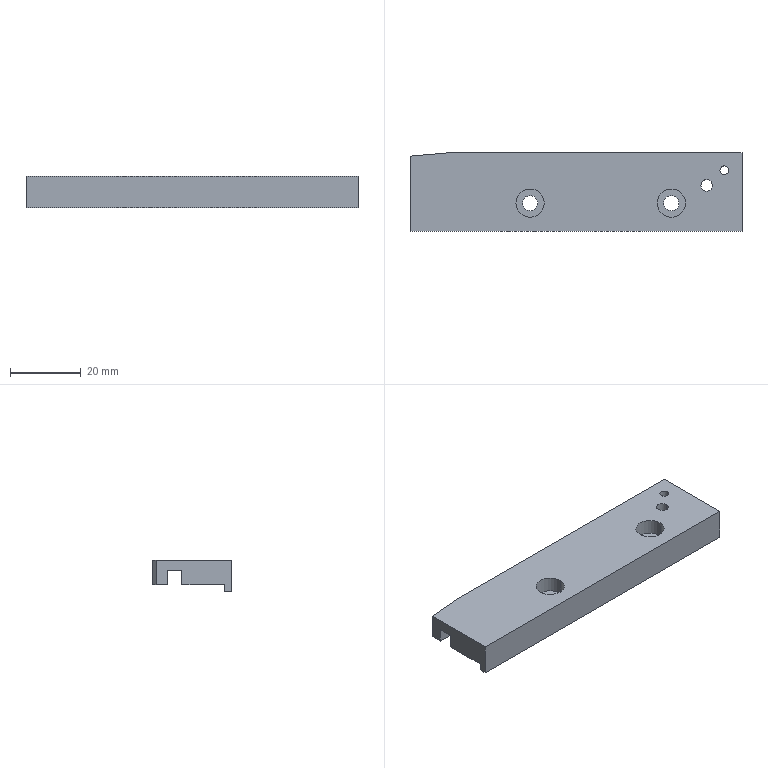Part | NX | features BREP 1 | 1 solid | 29 faces | box 94 x 22.3 x 9 mm | volume 12915 mm3 | plane 17 | cylinder 12 | commonest cylinder face diameters 4.3 x4 8 x4 2.5 x2 3.3 x2
STEP:
#1=CARTESIAN_POINT('',(33.75,6.15,4.));
#2=VERTEX_POINT('',#1);
#3=CARTESIAN_POINT('',(36.25,6.15,4.));
#4=VERTEX_POINT('',#3);
#5=CARTESIAN_POINT('',(35.,6.15,4.));
#6=DIRECTION('',(0.,0.,1.));
#7=DIRECTION('',(1.,0.,0.));
#8=AXIS2_PLACEMENT_3D('',#5,#6,#7);
#9=CIRCLE('',#8,1.25);
#10=EDGE_CURVE('',#2,#4,#9,.T.);
#11=ORIENTED_EDGE('',*,*,#10,.F.);
#12=CARTESIAN_POINT('',(33.75,6.15,7.));
#13=VERTEX_POINT('',#12);
#14=CARTESIAN_POINT('',(33.75,6.15,7.));
#15=DIRECTION('',(0.,0.,1.));
#16=VECTOR('',#15,1000.);
#17=LINE('',#14,#16);
#18=EDGE_CURVE('',#13,#2,#17,.F.);
#19=ORIENTED_EDGE('',*,*,#18,.F.);
#20=CARTESIAN_POINT('',(36.25,6.15,7.));
#21=VERTEX_POINT('',#20);
#22=CARTESIAN_POINT('',(35.,6.15,7.));
#23=DIRECTION('',(0.,0.,1.));
#24=DIRECTION('',(1.,0.,0.));
#25=AXIS2_PLACEMENT_3D('',#22,#23,#24);
#26=CIRCLE('',#25,1.25);
#27=EDGE_CURVE('',#13,#21,#26,.T.);
#28=ORIENTED_EDGE('',*,*,#27,.T.);
#29=CARTESIAN_POINT('',(36.25,6.15,7.));
#30=DIRECTION('',(0.,0.,1.));
#31=VECTOR('',#30,1000.);
#32=LINE('',#29,#31);
#33=EDGE_CURVE('',#21,#4,#32,.F.);
#34=ORIENTED_EDGE('',*,*,#33,.T.);
#35=EDGE_LOOP('',(#11,#19,#28,#34));
#36=FACE_BOUND('',#35,.T.);
#37=CARTESIAN_POINT('',(35.,6.15,7.));
#38=DIRECTION('',(0.,0.,1.));
#39=DIRECTION('',(1.,0.,0.));
#40=AXIS2_PLACEMENT_3D('',#37,#38,#39);
#41=CYLINDRICAL_SURFACE('',#40,1.25);
#42=ADVANCED_FACE('',(#36),#41,.F.);
#43=CARTESIAN_POINT('',(31.65,1.85,0.));
#44=VERTEX_POINT('',#43);
#45=CARTESIAN_POINT('',(28.35,1.85,0.));
#46=VERTEX_POINT('',#45);
#47=CARTESIAN_POINT('',(30.,1.85,0.));
#48=DIRECTION('',(0.,0.,-1.));
#49=DIRECTION('',(-1.,0.,0.));
#50=AXIS2_PLACEMENT_3D('',#47,#48,#49);
#51=CIRCLE('',#50,1.65);
#52=EDGE_CURVE('',#44,#46,#51,.T.);
#53=ORIENTED_EDGE('',*,*,#52,.T.);
#54=CARTESIAN_POINT('',(28.35,1.85,7.));
#55=VERTEX_POINT('',#54);
#56=CARTESIAN_POINT('',(28.35,1.85,7.));
#57=DIRECTION('',(0.,0.,1.));
#58=VECTOR('',#57,1000.);
#59=LINE('',#56,#58);
#60=EDGE_CURVE('',#55,#46,#59,.F.);
#61=ORIENTED_EDGE('',*,*,#60,.F.);
#62=CARTESIAN_POINT('',(31.65,1.85,7.));
#63=VERTEX_POINT('',#62);
#64=CARTESIAN_POINT('',(30.,1.85,7.));
#65=DIRECTION('',(0.,0.,1.));
#66=DIRECTION('',(1.,0.,0.));
#67=AXIS2_PLACEMENT_3D('',#64,#65,#66);
#68=CIRCLE('',#67,1.65);
#69=EDGE_CURVE('',#55,#63,#68,.T.);
#70=ORIENTED_EDGE('',*,*,#69,.T.);
#71=CARTESIAN_POINT('',(31.65,1.85,7.));
#72=DIRECTION('',(0.,0.,1.));
#73=VECTOR('',#72,1000.);
#74=LINE('',#71,#73);
#75=EDGE_CURVE('',#63,#44,#74,.F.);
#76=ORIENTED_EDGE('',*,*,#75,.T.);
#77=EDGE_LOOP('',(#53,#61,#70,#76));
#78=FACE_BOUND('',#77,.T.);
#79=CARTESIAN_POINT('',(30.,1.85,7.));
#80=DIRECTION('',(0.,0.,1.));
#81=DIRECTION('',(1.,0.,0.));
#82=AXIS2_PLACEMENT_3D('',#79,#80,#81);
#83=CYLINDRICAL_SURFACE('',#82,1.65);
#84=ADVANCED_FACE('',(#78),#83,.F.);
#85=CARTESIAN_POINT('',(16.,-3.15,2.6));
#86=VERTEX_POINT('',#85);
#87=CARTESIAN_POINT('',(24.,-3.15,2.6));
#88=VERTEX_POINT('',#87);
#89=CARTESIAN_POINT('',(20.,-3.15,2.6));
#90=DIRECTION('',(0.,0.,1.));
#91=DIRECTION('',(1.,0.,0.));
#92=AXIS2_PLACEMENT_3D('',#89,#90,#91);
#93=CIRCLE('',#92,4.);
#94=EDGE_CURVE('',#86,#88,#93,.T.);
#95=ORIENTED_EDGE('',*,*,#94,.F.);
#96=CARTESIAN_POINT('',(16.,-3.15,7.));
#97=VERTEX_POINT('',#96);
#98=CARTESIAN_POINT('',(16.,-3.15,7.));
#99=DIRECTION('',(0.,0.,1.));
#100=VECTOR('',#99,1000.);
#101=LINE('',#98,#100);
#102=EDGE_CURVE('',#97,#86,#101,.F.);
#103=ORIENTED_EDGE('',*,*,#102,.F.);
#104=CARTESIAN_POINT('',(24.,-3.15,7.));
#105=VERTEX_POINT('',#104);
#106=CARTESIAN_POINT('',(20.,-3.15,7.));
#107=DIRECTION('',(0.,0.,1.));
#108=DIRECTION('',(1.,0.,0.));
#109=AXIS2_PLACEMENT_3D('',#106,#107,#108);
#110=CIRCLE('',#109,4.);
#111=EDGE_CURVE('',#97,#105,#110,.T.);
#112=ORIENTED_EDGE('',*,*,#111,.T.);
#113=CARTESIAN_POINT('',(24.,-3.15,7.));
#114=DIRECTION('',(0.,0.,1.));
#115=VECTOR('',#114,1000.);
#116=LINE('',#113,#115);
#117=EDGE_CURVE('',#105,#88,#116,.F.);
#118=ORIENTED_EDGE('',*,*,#117,.T.);
#119=EDGE_LOOP('',(#95,#103,#112,#118));
#120=FACE_BOUND('',#119,.T.);
#121=CARTESIAN_POINT('',(20.,-3.15,7.));
#122=DIRECTION('',(0.,0.,1.));
#123=DIRECTION('',(1.,0.,0.));
#124=AXIS2_PLACEMENT_3D('',#121,#122,#123);
#125=CYLINDRICAL_SURFACE('',#124,4.);
#126=ADVANCED_FACE('',(#120),#125,.F.);
#127=CARTESIAN_POINT('',(17.85,-3.15,0.));
#128=VERTEX_POINT('',#127);
#129=CARTESIAN_POINT('',(22.15,-3.15,0.));
#130=VERTEX_POINT('',#129);
#131=CARTESIAN_POINT('',(20.,-3.15,0.));
#132=DIRECTION('',(0.,0.,1.));
#133=DIRECTION('',(1.,0.,0.));
#134=AXIS2_PLACEMENT_3D('',#131,#132,#133);
#135=CIRCLE('',#134,2.15);
#136=EDGE_CURVE('',#128,#130,#135,.T.);
#137=ORIENTED_EDGE('',*,*,#136,.F.);
#138=CARTESIAN_POINT('',(17.85,-3.15,2.6));
#139=VERTEX_POINT('',#138);
#140=CARTESIAN_POINT('',(17.85,-3.15,7.));
#141=DIRECTION('',(0.,0.,1.));
#142=VECTOR('',#141,1000.);
#143=LINE('',#140,#142);
#144=EDGE_CURVE('',#139,#128,#143,.F.);
#145=ORIENTED_EDGE('',*,*,#144,.F.);
#146=CARTESIAN_POINT('',(22.15,-3.15,2.6));
#147=VERTEX_POINT('',#146);
#148=CARTESIAN_POINT('',(20.,-3.15,2.6));
#149=DIRECTION('',(0.,0.,1.));
#150=DIRECTION('',(1.,0.,0.));
#151=AXIS2_PLACEMENT_3D('',#148,#149,#150);
#152=CIRCLE('',#151,2.15);
#153=EDGE_CURVE('',#139,#147,#152,.T.);
#154=ORIENTED_EDGE('',*,*,#153,.T.);
#155=CARTESIAN_POINT('',(22.15,-3.15,7.));
#156=DIRECTION('',(0.,0.,1.));
#157=VECTOR('',#156,1000.);
#158=LINE('',#155,#157);
#159=EDGE_CURVE('',#147,#130,#158,.F.);
#160=ORIENTED_EDGE('',*,*,#159,.T.);
#161=EDGE_LOOP('',(#137,#145,#154,#160));
#162=FACE_BOUND('',#161,.T.);
#163=CARTESIAN_POINT('',(20.,-3.15,7.));
#164=DIRECTION('',(0.,0.,1.));
#165=DIRECTION('',(1.,0.,0.));
#166=AXIS2_PLACEMENT_3D('',#163,#164,#165);
#167=CYLINDRICAL_SURFACE('',#166,2.15);
#168=ADVANCED_FACE('',(#162),#167,.F.);
#169=CARTESIAN_POINT('',(-24.,-3.15,2.6));
#170=VERTEX_POINT('',#169);
#171=CARTESIAN_POINT('',(-16.,-3.15,2.6));
#172=VERTEX_POINT('',#171);
#173=CARTESIAN_POINT('',(-20.,-3.15,2.6));
#174=DIRECTION('',(0.,0.,1.));
#175=DIRECTION('',(1.,0.,0.));
#176=AXIS2_PLACEMENT_3D('',#173,#174,#175);
#177=CIRCLE('',#176,4.);
#178=EDGE_CURVE('',#170,#172,#177,.T.);
#179=ORIENTED_EDGE('',*,*,#178,.F.);
#180=CARTESIAN_POINT('',(-24.,-3.15,7.));
#181=VERTEX_POINT('',#180);
#182=CARTESIAN_POINT('',(-24.,-3.15,7.));
#183=DIRECTION('',(0.,0.,1.));
#184=VECTOR('',#183,1000.);
#185=LINE('',#182,#184);
#186=EDGE_CURVE('',#181,#170,#185,.F.);
#187=ORIENTED_EDGE('',*,*,#186,.F.);
#188=CARTESIAN_POINT('',(-16.,-3.15,7.));
#189=VERTEX_POINT('',#188);
#190=CARTESIAN_POINT('',(-20.,-3.15,7.));
#191=DIRECTION('',(0.,0.,1.));
#192=DIRECTION('',(1.,0.,0.));
#193=AXIS2_PLACEMENT_3D('',#190,#191,#192);
#194=CIRCLE('',#193,4.);
#195=EDGE_CURVE('',#181,#189,#194,.T.);
#196=ORIENTED_EDGE('',*,*,#195,.T.);
#197=CARTESIAN_POINT('',(-16.,-3.15,7.));
#198=DIRECTION('',(0.,0.,1.));
#199=VECTOR('',#198,1000.);
#200=LINE('',#197,#199);
#201=EDGE_CURVE('',#189,#172,#200,.F.);
#202=ORIENTED_EDGE('',*,*,#201,.T.);
#203=EDGE_LOOP('',(#179,#187,#196,#202));
#204=FACE_BOUND('',#203,.T.);
#205=CARTESIAN_POINT('',(-20.,-3.15,7.));
#206=DIRECTION('',(0.,0.,1.));
#207=DIRECTION('',(1.,0.,0.));
#208=AXIS2_PLACEMENT_3D('',#205,#206,#207);
#209=CYLINDRICAL_SURFACE('',#208,4.);
#210=ADVANCED_FACE('',(#204),#209,.F.);
#211=CARTESIAN_POINT('',(-22.15,-3.15,0.));
#212=VERTEX_POINT('',#211);
#213=CARTESIAN_POINT('',(-17.85,-3.15,0.));
#214=VERTEX_POINT('',#213);
#215=CARTESIAN_POINT('',(-20.,-3.15,0.));
#216=DIRECTION('',(0.,0.,1.));
#217=DIRECTION('',(1.,0.,0.));
#218=AXIS2_PLACEMENT_3D('',#215,#216,#217);
#219=CIRCLE('',#218,2.15);
#220=EDGE_CURVE('',#212,#214,#219,.T.);
#221=ORIENTED_EDGE('',*,*,#220,.F.);
#222=CARTESIAN_POINT('',(-22.15,-3.15,2.6));
#223=VERTEX_POINT('',#222);
#224=CARTESIAN_POINT('',(-22.15,-3.15,7.));
#225=DIRECTION('',(0.,0.,1.));
#226=VECTOR('',#225,1000.);
#227=LINE('',#224,#226);
#228=EDGE_CURVE('',#223,#212,#227,.F.);
#229=ORIENTED_EDGE('',*,*,#228,.F.);
#230=CARTESIAN_POINT('',(-17.85,-3.15,2.6));
#231=VERTEX_POINT('',#230);
#232=CARTESIAN_POINT('',(-20.,-3.15,2.6));
#233=DIRECTION('',(0.,0.,1.));
#234=DIRECTION('',(1.,0.,0.));
#235=AXIS2_PLACEMENT_3D('',#232,#233,#234);
#236=CIRCLE('',#235,2.15);
#237=EDGE_CURVE('',#223,#231,#236,.T.);
#238=ORIENTED_EDGE('',*,*,#237,.T.);
#239=CARTESIAN_POINT('',(-17.85,-3.15,7.));
#240=DIRECTION('',(0.,0.,1.));
#241=VECTOR('',#240,1000.);
#242=LINE('',#239,#241);
#243=EDGE_CURVE('',#231,#214,#242,.F.);
#244=ORIENTED_EDGE('',*,*,#243,.T.);
#245=EDGE_LOOP('',(#221,#229,#238,#244));
#246=FACE_BOUND('',#245,.T.);
#247=CARTESIAN_POINT('',(-20.,-3.15,7.));
#248=DIRECTION('',(0.,0.,1.));
#249=DIRECTION('',(1.,0.,0.));
#250=AXIS2_PLACEMENT_3D('',#247,#248,#249);
#251=CYLINDRICAL_SURFACE('',#250,2.15);
#252=ADVANCED_FACE('',(#246),#251,.F.);
#253=CARTESIAN_POINT('',(-54.,6.85,0.));
#254=VERTEX_POINT('',#253);
#255=CARTESIAN_POINT('',(33.964,6.85,0.));
#256=VERTEX_POINT('',#255);
#257=CARTESIAN_POINT('',(-64.957,6.85,0.));
#258=DIRECTION('',(1.,0.,0.));
#259=VECTOR('',#258,1000.);
#260=LINE('',#257,#259);
#261=EDGE_CURVE('',#254,#256,#260,.T.);
#262=ORIENTED_EDGE('',*,*,#261,.T.);
#263=CARTESIAN_POINT('',(33.964,6.85,4.));
#264=VERTEX_POINT('',#263);
#265=CARTESIAN_POINT('',(33.964,6.85,7.));
#266=DIRECTION('',(0.,0.,1.));
#267=VECTOR('',#266,1000.);
#268=LINE('',#265,#267);
#269=EDGE_CURVE('',#256,#264,#268,.T.);
#270=ORIENTED_EDGE('',*,*,#269,.T.);
#271=CARTESIAN_POINT('',(-54.,6.85,4.));
#272=VERTEX_POINT('',#271);
#273=CARTESIAN_POINT('',(-64.957,6.85,4.));
#274=DIRECTION('',(1.,0.,0.));
#275=VECTOR('',#274,1000.);
#276=LINE('',#273,#275);
#277=EDGE_CURVE('',#272,#264,#276,.T.);
#278=ORIENTED_EDGE('',*,*,#277,.F.);
#279=CARTESIAN_POINT('',(-54.,6.85,7.));
#280=DIRECTION('',(0.,0.,1.));
#281=VECTOR('',#280,1000.);
#282=LINE('',#279,#281);
#283=EDGE_CURVE('',#254,#272,#282,.T.);
#284=ORIENTED_EDGE('',*,*,#283,.F.);
#285=EDGE_LOOP('',(#262,#270,#278,#284));
#286=FACE_BOUND('',#285,.T.);
#287=CARTESIAN_POINT('',(-64.957,6.85,4.));
#288=DIRECTION('',(0.,1.,0.));
#289=DIRECTION('',(1.,0.,0.));
#290=AXIS2_PLACEMENT_3D('',#287,#288,#289);
#291=PLANE('',#290);
#292=ADVANCED_FACE('',(#286),#291,.F.);
#293=CARTESIAN_POINT('',(36.036,6.85,0.));
#294=VERTEX_POINT('',#293);
#295=CARTESIAN_POINT('',(35.,6.15,0.));
#296=DIRECTION('',(0.,0.,-1.));
#297=DIRECTION('',(-1.,0.,0.));
#298=AXIS2_PLACEMENT_3D('',#295,#296,#297);
#299=CIRCLE('',#298,1.25);
#300=EDGE_CURVE('',#256,#294,#299,.T.);
#301=ORIENTED_EDGE('',*,*,#300,.F.);
#302=ORIENTED_EDGE('',*,*,#261,.F.);
#303=CARTESIAN_POINT('',(-54.,10.15,0.));
#304=VERTEX_POINT('',#303);
#305=CARTESIAN_POINT('',(-54.,-11.15,0.));
#306=DIRECTION('',(0.,-1.,0.));
#307=VECTOR('',#306,1000.);
#308=LINE('',#305,#307);
#309=EDGE_CURVE('',#304,#254,#308,.T.);
#310=ORIENTED_EDGE('',*,*,#309,.F.);
#311=CARTESIAN_POINT('',(-42.57,11.15,0.));
#312=VERTEX_POINT('',#311);
#313=CARTESIAN_POINT('',(-15.185,13.546,0.));
#314=DIRECTION('',(0.9962,0.08716,0.));
#315=VECTOR('',#314,1000.);
#316=LINE('',#313,#315);
#317=EDGE_CURVE('',#304,#312,#316,.T.);
#318=ORIENTED_EDGE('',*,*,#317,.T.);
#319=CARTESIAN_POINT('',(40.,11.15,0.));
#320=VERTEX_POINT('',#319);
#321=CARTESIAN_POINT('',(-40.,11.15,0.));
#322=DIRECTION('',(-1.,0.,0.));
#323=VECTOR('',#322,1000.);
#324=LINE('',#321,#323);
#325=EDGE_CURVE('',#320,#312,#324,.T.);
#326=ORIENTED_EDGE('',*,*,#325,.F.);
#327=CARTESIAN_POINT('',(40.,6.85,0.));
#328=VERTEX_POINT('',#327);
#329=CARTESIAN_POINT('',(40.,-11.15,0.));
#330=DIRECTION('',(0.,1.,0.));
#331=VECTOR('',#330,1000.);
#332=LINE('',#329,#331);
#333=EDGE_CURVE('',#328,#320,#332,.T.);
#334=ORIENTED_EDGE('',*,*,#333,.F.);
#335=CARTESIAN_POINT('',(-64.957,6.85,0.));
#336=DIRECTION('',(1.,0.,0.));
#337=VECTOR('',#336,1000.);
#338=LINE('',#335,#337);
#339=EDGE_CURVE('',#294,#328,#338,.T.);
#340=ORIENTED_EDGE('',*,*,#339,.F.);
#341=EDGE_LOOP('',(#301,#302,#310,#318,#326,#334,#340));
#342=FACE_BOUND('',#341,.T.);
#343=CARTESIAN_POINT('',(0.,0.,0.));
#344=DIRECTION('',(0.,0.,-1.));
#345=DIRECTION('',(0.,-1.,0.));
#346=AXIS2_PLACEMENT_3D('',#343,#344,#345);
#347=PLANE('',#346);
#348=ADVANCED_FACE('',(#342),#347,.T.);
#349=CARTESIAN_POINT('',(40.,2.85,4.));
#350=VERTEX_POINT('',#349);
#351=CARTESIAN_POINT('',(40.,6.85,4.));
#352=VERTEX_POINT('',#351);
#353=CARTESIAN_POINT('',(40.,-11.15,4.));
#354=DIRECTION('',(0.,1.,0.));
#355=VECTOR('',#354,1000.);
#356=LINE('',#353,#355);
#357=EDGE_CURVE('',#350,#352,#356,.T.);
#358=ORIENTED_EDGE('',*,*,#357,.T.);
#359=CARTESIAN_POINT('',(40.,6.85,7.));
#360=DIRECTION('',(0.,0.,-1.));
#361=VECTOR('',#360,1000.);
#362=LINE('',#359,#361);
#363=EDGE_CURVE('',#352,#328,#362,.T.);
#364=ORIENTED_EDGE('',*,*,#363,.T.);
#365=ORIENTED_EDGE('',*,*,#333,.T.);
#366=CARTESIAN_POINT('',(40.,11.15,7.));
#367=VERTEX_POINT('',#366);
#368=CARTESIAN_POINT('',(40.,11.15,7.));
#369=DIRECTION('',(0.,0.,-1.));
#370=VECTOR('',#369,1000.);
#371=LINE('',#368,#370);
#372=EDGE_CURVE('',#367,#320,#371,.T.);
#373=ORIENTED_EDGE('',*,*,#372,.F.);
#374=CARTESIAN_POINT('',(40.,-11.15,7.));
#375=VERTEX_POINT('',#374);
#376=CARTESIAN_POINT('',(40.,-11.15,7.));
#377=DIRECTION('',(0.,1.,0.));
#378=VECTOR('',#377,1000.);
#379=LINE('',#376,#378);
#380=EDGE_CURVE('',#375,#367,#379,.T.);
#381=ORIENTED_EDGE('',*,*,#380,.F.);
#382=CARTESIAN_POINT('',(40.,-11.15,-2.));
#383=VERTEX_POINT('',#382);
#384=CARTESIAN_POINT('',(40.,-11.15,7.));
#385=DIRECTION('',(0.,0.,-1.));
#386=VECTOR('',#385,1000.);
#387=LINE('',#384,#386);
#388=EDGE_CURVE('',#375,#383,#387,.T.);
#389=ORIENTED_EDGE('',*,*,#388,.T.);
#390=CARTESIAN_POINT('',(40.,-9.15,-2.));
#391=VERTEX_POINT('',#390);
#392=CARTESIAN_POINT('',(40.,-11.15,-2.));
#393=DIRECTION('',(0.,-1.,0.));
#394=VECTOR('',#393,1000.);
#395=LINE('',#392,#394);
#396=EDGE_CURVE('',#391,#383,#395,.T.);
#397=ORIENTED_EDGE('',*,*,#396,.F.);
#398=CARTESIAN_POINT('',(40.,-9.15,0.));
#399=VERTEX_POINT('',#398);
#400=CARTESIAN_POINT('',(40.,-9.15,-2.));
#401=DIRECTION('',(0.,0.,1.));
#402=VECTOR('',#401,1000.);
#403=LINE('',#400,#402);
#404=EDGE_CURVE('',#391,#399,#403,.T.);
#405=ORIENTED_EDGE('',*,*,#404,.T.);
#406=CARTESIAN_POINT('',(40.,2.85,0.));
#407=VERTEX_POINT('',#406);
#408=CARTESIAN_POINT('',(40.,-11.15,0.));
#409=DIRECTION('',(0.,1.,0.));
#410=VECTOR('',#409,1000.);
#411=LINE('',#408,#410);
#412=EDGE_CURVE('',#399,#407,#411,.T.);
#413=ORIENTED_EDGE('',*,*,#412,.T.);
#414=CARTESIAN_POINT('',(40.,2.85,7.));
#415=DIRECTION('',(0.,0.,1.));
#416=VECTOR('',#415,1000.);
#417=LINE('',#414,#416);
#418=EDGE_CURVE('',#407,#350,#417,.T.);
#419=ORIENTED_EDGE('',*,*,#418,.T.);
#420=EDGE_LOOP('',(#358,#364,#365,#373,#381,#389,#397,#405,#413,#419));
#421=FACE_BOUND('',#420,.T.);
#422=CARTESIAN_POINT('',(40.,-11.15,7.));
#423=DIRECTION('',(-1.,0.,0.));
#424=DIRECTION('',(0.,0.,1.));
#425=AXIS2_PLACEMENT_3D('',#422,#423,#424);
#426=PLANE('',#425);
#427=ADVANCED_FACE('',(#421),#426,.F.);
#428=ORIENTED_EDGE('',*,*,#325,.T.);
#429=CARTESIAN_POINT('',(-42.57,11.15,7.));
#430=VERTEX_POINT('',#429);
#431=CARTESIAN_POINT('',(-42.57,11.15,7.));
#432=DIRECTION('',(0.,0.,1.));
#433=VECTOR('',#432,1000.);
#434=LINE('',#431,#433);
#435=EDGE_CURVE('',#312,#430,#434,.T.);
#436=ORIENTED_EDGE('',*,*,#435,.T.);
#437=CARTESIAN_POINT('',(-40.,11.15,7.));
#438=DIRECTION('',(-1.,0.,0.));
#439=VECTOR('',#438,1000.);
#440=LINE('',#437,#439);
#441=EDGE_CURVE('',#367,#430,#440,.T.);
#442=ORIENTED_EDGE('',*,*,#441,.F.);
#443=ORIENTED_EDGE('',*,*,#372,.T.);
#444=EDGE_LOOP('',(#428,#436,#442,#443));
#445=FACE_BOUND('',#444,.T.);
#446=CARTESIAN_POINT('',(-40.,11.15,7.));
#447=DIRECTION('',(0.,-1.,0.));
#448=DIRECTION('',(0.,0.,-1.));
#449=AXIS2_PLACEMENT_3D('',#446,#447,#448);
#450=PLANE('',#449);
#451=ADVANCED_FACE('',(#445),#450,.F.);
#452=ORIENTED_EDGE('',*,*,#309,.T.);
#453=ORIENTED_EDGE('',*,*,#283,.T.);
#454=CARTESIAN_POINT('',(-54.,2.85,4.));
#455=VERTEX_POINT('',#454);
#456=CARTESIAN_POINT('',(-54.,-11.15,4.));
#457=DIRECTION('',(0.,-1.,0.));
#458=VECTOR('',#457,1000.);
#459=LINE('',#456,#458);
#460=EDGE_CURVE('',#272,#455,#459,.T.);
#461=ORIENTED_EDGE('',*,*,#460,.T.);
#462=CARTESIAN_POINT('',(-54.,2.85,0.));
#463=VERTEX_POINT('',#462);
#464=CARTESIAN_POINT('',(-54.,2.85,7.));
#465=DIRECTION('',(0.,0.,-1.));
#466=VECTOR('',#465,1000.);
#467=LINE('',#464,#466);
#468=EDGE_CURVE('',#455,#463,#467,.T.);
#469=ORIENTED_EDGE('',*,*,#468,.T.);
#470=CARTESIAN_POINT('',(-54.,-9.15,0.));
#471=VERTEX_POINT('',#470);
#472=CARTESIAN_POINT('',(-54.,-11.15,0.));
#473=DIRECTION('',(0.,-1.,0.));
#474=VECTOR('',#473,1000.);
#475=LINE('',#472,#474);
#476=EDGE_CURVE('',#463,#471,#475,.T.);
#477=ORIENTED_EDGE('',*,*,#476,.T.);
#478=CARTESIAN_POINT('',(-54.,-9.15,-2.));
#479=VERTEX_POINT('',#478);
#480=CARTESIAN_POINT('',(-54.,-9.15,-2.));
#481=DIRECTION('',(0.,0.,1.));
#482=VECTOR('',#481,1000.);
#483=LINE('',#480,#482);
#484=EDGE_CURVE('',#479,#471,#483,.T.);
#485=ORIENTED_EDGE('',*,*,#484,.F.);
#486=CARTESIAN_POINT('',(-54.,-11.15,-2.));
#487=VERTEX_POINT('',#486);
#488=CARTESIAN_POINT('',(-54.,-11.15,-2.));
#489=DIRECTION('',(0.,1.,0.));
#490=VECTOR('',#489,1000.);
#491=LINE('',#488,#490);
#492=EDGE_CURVE('',#487,#479,#491,.T.);
#493=ORIENTED_EDGE('',*,*,#492,.F.);
#494=CARTESIAN_POINT('',(-54.,-11.15,7.));
#495=VERTEX_POINT('',#494);
#496=CARTESIAN_POINT('',(-54.,-11.15,7.));
#497=DIRECTION('',(0.,0.,-1.));
#498=VECTOR('',#497,1000.);
#499=LINE('',#496,#498);
#500=EDGE_CURVE('',#495,#487,#499,.T.);
#501=ORIENTED_EDGE('',*,*,#500,.F.);
#502=CARTESIAN_POINT('',(-54.,10.15,7.));
#503=VERTEX_POINT('',#502);
#504=CARTESIAN_POINT('',(-54.,-11.15,7.));
#505=DIRECTION('',(0.,-1.,0.));
#506=VECTOR('',#505,1000.);
#507=LINE('',#504,#506);
#508=EDGE_CURVE('',#503,#495,#507,.T.);
#509=ORIENTED_EDGE('',*,*,#508,.F.);
#510=CARTESIAN_POINT('',(-54.,10.15,7.));
#511=DIRECTION('',(0.,0.,-1.));
#512=VECTOR('',#511,1000.);
#513=LINE('',#510,#512);
#514=EDGE_CURVE('',#503,#304,#513,.T.);
#515=ORIENTED_EDGE('',*,*,#514,.T.);
#516=EDGE_LOOP('',(#452,#453,#461,#469,#477,#485,#493,#501,#509,#515));
#517=FACE_BOUND('',#516,.T.);
#518=CARTESIAN_POINT('',(-54.,-11.15,7.));
#519=DIRECTION('',(1.,0.,0.));
#520=DIRECTION('',(0.,1.,0.));
#521=AXIS2_PLACEMENT_3D('',#518,#519,#520);
#522=PLANE('',#521);
#523=ADVANCED_FACE('',(#517),#522,.F.);
#524=ORIENTED_EDGE('',*,*,#500,.T.);
#525=CARTESIAN_POINT('',(-40.,-11.15,-2.));
#526=DIRECTION('',(-1.,0.,0.));
#527=VECTOR('',#526,1000.);
#528=LINE('',#525,#527);
#529=EDGE_CURVE('',#383,#487,#528,.T.);
#530=ORIENTED_EDGE('',*,*,#529,.F.);
#531=ORIENTED_EDGE('',*,*,#388,.F.);
#532=CARTESIAN_POINT('',(-40.,-11.15,7.));
#533=DIRECTION('',(1.,0.,0.));
#534=VECTOR('',#533,1000.);
#535=LINE('',#532,#534);
#536=EDGE_CURVE('',#495,#375,#535,.T.);
#537=ORIENTED_EDGE('',*,*,#536,.F.);
#538=EDGE_LOOP('',(#524,#530,#531,#537));
#539=FACE_BOUND('',#538,.T.);
#540=CARTESIAN_POINT('',(-40.,-11.15,7.));
#541=DIRECTION('',(0.,1.,0.));
#542=DIRECTION('',(1.,0.,0.));
#543=AXIS2_PLACEMENT_3D('',#540,#541,#542);
#544=PLANE('',#543);
#545=ADVANCED_FACE('',(#539),#544,.F.);
#546=ORIENTED_EDGE('',*,*,#441,.T.);
#547=CARTESIAN_POINT('',(-54.,10.15,7.));
#548=DIRECTION('',(-0.9962,-0.08716,0.));
#549=VECTOR('',#548,1000.);
#550=LINE('',#547,#549);
#551=EDGE_CURVE('',#430,#503,#550,.T.);
#552=ORIENTED_EDGE('',*,*,#551,.T.);
#553=ORIENTED_EDGE('',*,*,#508,.T.);
#554=ORIENTED_EDGE('',*,*,#536,.T.);
#555=ORIENTED_EDGE('',*,*,#380,.T.);
#556=EDGE_LOOP('',(#546,#552,#553,#554,#555));
#557=FACE_BOUND('',#556,.T.);
#558=CARTESIAN_POINT('',(35.,6.15,7.));
#559=DIRECTION('',(0.,0.,1.));
#560=DIRECTION('',(1.,0.,0.));
#561=AXIS2_PLACEMENT_3D('',#558,#559,#560);
#562=CIRCLE('',#561,1.25);
#563=EDGE_CURVE('',#21,#13,#562,.T.);
#564=ORIENTED_EDGE('',*,*,#563,.F.);
#565=ORIENTED_EDGE('',*,*,#27,.F.);
#566=EDGE_LOOP('',(#564,#565));
#567=FACE_BOUND('',#566,.T.);
#568=CARTESIAN_POINT('',(30.,1.85,7.));
#569=DIRECTION('',(0.,0.,1.));
#570=DIRECTION('',(1.,0.,0.));
#571=AXIS2_PLACEMENT_3D('',#568,#569,#570);
#572=CIRCLE('',#571,1.65);
#573=EDGE_CURVE('',#63,#55,#572,.T.);
#574=ORIENTED_EDGE('',*,*,#573,.F.);
#575=ORIENTED_EDGE('',*,*,#69,.F.);
#576=EDGE_LOOP('',(#574,#575));
#577=FACE_BOUND('',#576,.T.);
#578=CARTESIAN_POINT('',(20.,-3.15,7.));
#579=DIRECTION('',(0.,0.,1.));
#580=DIRECTION('',(1.,0.,0.));
#581=AXIS2_PLACEMENT_3D('',#578,#579,#580);
#582=CIRCLE('',#581,4.);
#583=EDGE_CURVE('',#105,#97,#582,.T.);
#584=ORIENTED_EDGE('',*,*,#583,.F.);
#585=ORIENTED_EDGE('',*,*,#111,.F.);
#586=EDGE_LOOP('',(#584,#585));
#587=FACE_BOUND('',#586,.T.);
#588=CARTESIAN_POINT('',(-20.,-3.15,7.));
#589=DIRECTION('',(0.,0.,1.));
#590=DIRECTION('',(1.,0.,0.));
#591=AXIS2_PLACEMENT_3D('',#588,#589,#590);
#592=CIRCLE('',#591,4.);
#593=EDGE_CURVE('',#189,#181,#592,.T.);
#594=ORIENTED_EDGE('',*,*,#593,.F.);
#595=ORIENTED_EDGE('',*,*,#195,.F.);
#596=EDGE_LOOP('',(#594,#595));
#597=FACE_BOUND('',#596,.T.);
#598=CARTESIAN_POINT('',(0.,0.,7.));
#599=DIRECTION('',(0.,0.,-1.));
#600=DIRECTION('',(0.,-1.,0.));
#601=AXIS2_PLACEMENT_3D('',#598,#599,#600);
#602=PLANE('',#601);
#603=ADVANCED_FACE('',(#557,#567,#577,#587,#597),#602,.F.);
#604=CARTESIAN_POINT('',(31.312,2.85,0.));
#605=VERTEX_POINT('',#604);
#606=CARTESIAN_POINT('',(-64.957,2.85,0.));
#607=DIRECTION('',(-1.,0.,0.));
#608=VECTOR('',#607,1000.);
#609=LINE('',#606,#608);
#610=EDGE_CURVE('',#407,#605,#609,.T.);
#611=ORIENTED_EDGE('',*,*,#610,.F.);
#612=ORIENTED_EDGE('',*,*,#412,.F.);
#613=CARTESIAN_POINT('',(-40.,-9.15,0.));
#614=DIRECTION('',(1.,0.,0.));
#615=VECTOR('',#614,1000.);
#616=LINE('',#613,#615);
#617=EDGE_CURVE('',#471,#399,#616,.T.);
#618=ORIENTED_EDGE('',*,*,#617,.F.);
#619=ORIENTED_EDGE('',*,*,#476,.F.);
#620=CARTESIAN_POINT('',(28.688,2.85,0.));
#621=VERTEX_POINT('',#620);
#622=CARTESIAN_POINT('',(-64.957,2.85,0.));
#623=DIRECTION('',(-1.,0.,0.));
#624=VECTOR('',#623,1000.);
#625=LINE('',#622,#624);
#626=EDGE_CURVE('',#621,#463,#625,.T.);
#627=ORIENTED_EDGE('',*,*,#626,.F.);
#628=CARTESIAN_POINT('',(30.,1.85,0.));
#629=DIRECTION('',(0.,0.,-1.));
#630=DIRECTION('',(-1.,0.,0.));
#631=AXIS2_PLACEMENT_3D('',#628,#629,#630);
#632=CIRCLE('',#631,1.65);
#633=EDGE_CURVE('',#46,#621,#632,.T.);
#634=ORIENTED_EDGE('',*,*,#633,.F.);
#635=ORIENTED_EDGE('',*,*,#52,.F.);
#636=CARTESIAN_POINT('',(30.,1.85,0.));
#637=DIRECTION('',(0.,0.,-1.));
#638=DIRECTION('',(-1.,0.,0.));
#639=AXIS2_PLACEMENT_3D('',#636,#637,#638);
#640=CIRCLE('',#639,1.65);
#641=EDGE_CURVE('',#605,#44,#640,.T.);
#642=ORIENTED_EDGE('',*,*,#641,.F.);
#643=EDGE_LOOP('',(#611,#612,#618,#619,#627,#634,#635,#642));
#644=FACE_BOUND('',#643,.T.);
#645=CARTESIAN_POINT('',(20.,-3.15,0.));
#646=DIRECTION('',(0.,0.,1.));
#647=DIRECTION('',(1.,0.,0.));
#648=AXIS2_PLACEMENT_3D('',#645,#646,#647);
#649=CIRCLE('',#648,2.15);
#650=EDGE_CURVE('',#130,#128,#649,.T.);
#651=ORIENTED_EDGE('',*,*,#650,.T.);
#652=ORIENTED_EDGE('',*,*,#136,.T.);
#653=EDGE_LOOP('',(#651,#652));
#654=FACE_BOUND('',#653,.T.);
#655=CARTESIAN_POINT('',(-20.,-3.15,0.));
#656=DIRECTION('',(0.,0.,1.));
#657=DIRECTION('',(1.,0.,0.));
#658=AXIS2_PLACEMENT_3D('',#655,#656,#657);
#659=CIRCLE('',#658,2.15);
#660=EDGE_CURVE('',#214,#212,#659,.T.);
#661=ORIENTED_EDGE('',*,*,#660,.T.);
#662=ORIENTED_EDGE('',*,*,#220,.T.);
#663=EDGE_LOOP('',(#661,#662));
#664=FACE_BOUND('',#663,.T.);
#665=CARTESIAN_POINT('',(0.,0.,0.));
#666=DIRECTION('',(0.,0.,-1.));
#667=DIRECTION('',(0.,-1.,0.));
#668=AXIS2_PLACEMENT_3D('',#665,#666,#667);
#669=PLANE('',#668);
#670=ADVANCED_FACE('',(#644,#654,#664),#669,.T.);
#671=ORIENTED_EDGE('',*,*,#551,.F.);
#672=ORIENTED_EDGE('',*,*,#435,.F.);
#673=ORIENTED_EDGE('',*,*,#317,.F.);
#674=ORIENTED_EDGE('',*,*,#514,.F.);
#675=EDGE_LOOP('',(#671,#672,#673,#674));
#676=FACE_BOUND('',#675,.T.);
#677=CARTESIAN_POINT('',(-54.,10.15,7.));
#678=DIRECTION('',(0.08716,-0.9962,0.));
#679=DIRECTION('',(0.,0.,-1.));
#680=AXIS2_PLACEMENT_3D('',#677,#678,#679);
#681=PLANE('',#680);
#682=ADVANCED_FACE('',(#676),#681,.F.);
#683=ORIENTED_EDGE('',*,*,#228,.T.);
#684=ORIENTED_EDGE('',*,*,#660,.F.);
#685=ORIENTED_EDGE('',*,*,#243,.F.);
#686=CARTESIAN_POINT('',(-20.,-3.15,2.6));
#687=DIRECTION('',(0.,0.,1.));
#688=DIRECTION('',(1.,0.,0.));
#689=AXIS2_PLACEMENT_3D('',#686,#687,#688);
#690=CIRCLE('',#689,2.15);
#691=EDGE_CURVE('',#231,#223,#690,.T.);
#692=ORIENTED_EDGE('',*,*,#691,.T.);
#693=EDGE_LOOP('',(#683,#684,#685,#692));
#694=FACE_BOUND('',#693,.T.);
#695=CARTESIAN_POINT('',(-20.,-3.15,7.));
#696=DIRECTION('',(0.,0.,1.));
#697=DIRECTION('',(1.,0.,0.));
#698=AXIS2_PLACEMENT_3D('',#695,#696,#697);
#699=CYLINDRICAL_SURFACE('',#698,2.15);
#700=ADVANCED_FACE('',(#694),#699,.F.);
#701=CARTESIAN_POINT('',(-20.,-3.15,2.6));
#702=DIRECTION('',(0.,0.,1.));
#703=DIRECTION('',(1.,0.,0.));
#704=AXIS2_PLACEMENT_3D('',#701,#702,#703);
#705=CIRCLE('',#704,4.);
#706=EDGE_CURVE('',#172,#170,#705,.T.);
#707=ORIENTED_EDGE('',*,*,#706,.T.);
#708=ORIENTED_EDGE('',*,*,#178,.T.);
#709=EDGE_LOOP('',(#707,#708));
#710=FACE_BOUND('',#709,.T.);
#711=ORIENTED_EDGE('',*,*,#691,.F.);
#712=ORIENTED_EDGE('',*,*,#237,.F.);
#713=EDGE_LOOP('',(#711,#712));
#714=FACE_BOUND('',#713,.T.);
#715=CARTESIAN_POINT('',(-17.85,-3.15,2.6));
#716=DIRECTION('',(0.,0.,-1.));
#717=DIRECTION('',(0.,-1.,0.));
#718=AXIS2_PLACEMENT_3D('',#715,#716,#717);
#719=PLANE('',#718);
#720=ADVANCED_FACE('',(#710,#714),#719,.F.);
#721=ORIENTED_EDGE('',*,*,#186,.T.);
#722=ORIENTED_EDGE('',*,*,#706,.F.);
#723=ORIENTED_EDGE('',*,*,#201,.F.);
#724=ORIENTED_EDGE('',*,*,#593,.T.);
#725=EDGE_LOOP('',(#721,#722,#723,#724));
#726=FACE_BOUND('',#725,.T.);
#727=CARTESIAN_POINT('',(-20.,-3.15,7.));
#728=DIRECTION('',(0.,0.,1.));
#729=DIRECTION('',(1.,0.,0.));
#730=AXIS2_PLACEMENT_3D('',#727,#728,#729);
#731=CYLINDRICAL_SURFACE('',#730,4.);
#732=ADVANCED_FACE('',(#726),#731,.F.);
#733=ORIENTED_EDGE('',*,*,#617,.T.);
#734=ORIENTED_EDGE('',*,*,#404,.F.);
#735=CARTESIAN_POINT('',(-40.,-9.15,-2.));
#736=DIRECTION('',(1.,0.,0.));
#737=VECTOR('',#736,1000.);
#738=LINE('',#735,#737);
#739=EDGE_CURVE('',#479,#391,#738,.T.);
#740=ORIENTED_EDGE('',*,*,#739,.F.);
#741=ORIENTED_EDGE('',*,*,#484,.T.);
#742=EDGE_LOOP('',(#733,#734,#740,#741));
#743=FACE_BOUND('',#742,.T.);
#744=CARTESIAN_POINT('',(-40.,-9.15,-2.));
#745=DIRECTION('',(0.,-1.,0.));
#746=DIRECTION('',(-1.,0.,0.));
#747=AXIS2_PLACEMENT_3D('',#744,#745,#746);
#748=PLANE('',#747);
#749=ADVANCED_FACE('',(#743),#748,.F.);
#750=ORIENTED_EDGE('',*,*,#492,.T.);
#751=ORIENTED_EDGE('',*,*,#739,.T.);
#752=ORIENTED_EDGE('',*,*,#396,.T.);
#753=ORIENTED_EDGE('',*,*,#529,.T.);
#754=EDGE_LOOP('',(#750,#751,#752,#753));
#755=FACE_BOUND('',#754,.T.);
#756=CARTESIAN_POINT('',(0.,0.,-2.));
#757=DIRECTION('',(0.,0.,-1.));
#758=DIRECTION('',(0.,-1.,0.));
#759=AXIS2_PLACEMENT_3D('',#756,#757,#758);
#760=PLANE('',#759);
#761=ADVANCED_FACE('',(#755),#760,.T.);
#762=ORIENTED_EDGE('',*,*,#144,.T.);
#763=ORIENTED_EDGE('',*,*,#650,.F.);
#764=ORIENTED_EDGE('',*,*,#159,.F.);
#765=CARTESIAN_POINT('',(20.,-3.15,2.6));
#766=DIRECTION('',(0.,0.,1.));
#767=DIRECTION('',(1.,0.,0.));
#768=AXIS2_PLACEMENT_3D('',#765,#766,#767);
#769=CIRCLE('',#768,2.15);
#770=EDGE_CURVE('',#147,#139,#769,.T.);
#771=ORIENTED_EDGE('',*,*,#770,.T.);
#772=EDGE_LOOP('',(#762,#763,#764,#771));
#773=FACE_BOUND('',#772,.T.);
#774=CARTESIAN_POINT('',(20.,-3.15,7.));
#775=DIRECTION('',(0.,0.,1.));
#776=DIRECTION('',(1.,0.,0.));
#777=AXIS2_PLACEMENT_3D('',#774,#775,#776);
#778=CYLINDRICAL_SURFACE('',#777,2.15);
#779=ADVANCED_FACE('',(#773),#778,.F.);
#780=CARTESIAN_POINT('',(20.,-3.15,2.6));
#781=DIRECTION('',(0.,0.,1.));
#782=DIRECTION('',(1.,0.,0.));
#783=AXIS2_PLACEMENT_3D('',#780,#781,#782);
#784=CIRCLE('',#783,4.);
#785=EDGE_CURVE('',#88,#86,#784,.T.);
#786=ORIENTED_EDGE('',*,*,#785,.T.);
#787=ORIENTED_EDGE('',*,*,#94,.T.);
#788=EDGE_LOOP('',(#786,#787));
#789=FACE_BOUND('',#788,.T.);
#790=ORIENTED_EDGE('',*,*,#770,.F.);
#791=ORIENTED_EDGE('',*,*,#153,.F.);
#792=EDGE_LOOP('',(#790,#791));
#793=FACE_BOUND('',#792,.T.);
#794=CARTESIAN_POINT('',(22.15,-3.15,2.6));
#795=DIRECTION('',(0.,0.,-1.));
#796=DIRECTION('',(0.,-1.,0.));
#797=AXIS2_PLACEMENT_3D('',#794,#795,#796);
#798=PLANE('',#797);
#799=ADVANCED_FACE('',(#789,#793),#798,.F.);
#800=ORIENTED_EDGE('',*,*,#102,.T.);
#801=ORIENTED_EDGE('',*,*,#785,.F.);
#802=ORIENTED_EDGE('',*,*,#117,.F.);
#803=ORIENTED_EDGE('',*,*,#583,.T.);
#804=EDGE_LOOP('',(#800,#801,#802,#803));
#805=FACE_BOUND('',#804,.T.);
#806=CARTESIAN_POINT('',(20.,-3.15,7.));
#807=DIRECTION('',(0.,0.,1.));
#808=DIRECTION('',(1.,0.,0.));
#809=AXIS2_PLACEMENT_3D('',#806,#807,#808);
#810=CYLINDRICAL_SURFACE('',#809,4.);
#811=ADVANCED_FACE('',(#805),#810,.F.);
#812=ORIENTED_EDGE('',*,*,#60,.T.);
#813=ORIENTED_EDGE('',*,*,#633,.T.);
#814=CARTESIAN_POINT('',(28.688,2.85,4.));
#815=VERTEX_POINT('',#814);
#816=CARTESIAN_POINT('',(28.688,2.85,7.));
#817=DIRECTION('',(0.,0.,1.));
#818=VECTOR('',#817,1000.);
#819=LINE('',#816,#818);
#820=EDGE_CURVE('',#621,#815,#819,.T.);
#821=ORIENTED_EDGE('',*,*,#820,.T.);
#822=CARTESIAN_POINT('',(31.312,2.85,4.));
#823=VERTEX_POINT('',#822);
#824=CARTESIAN_POINT('',(30.,1.85,4.));
#825=DIRECTION('',(0.,0.,-1.));
#826=DIRECTION('',(1.,0.,0.));
#827=AXIS2_PLACEMENT_3D('',#824,#825,#826);
#828=CIRCLE('',#827,1.65);
#829=EDGE_CURVE('',#815,#823,#828,.T.);
#830=ORIENTED_EDGE('',*,*,#829,.T.);
#831=CARTESIAN_POINT('',(31.312,2.85,7.));
#832=DIRECTION('',(0.,0.,-1.));
#833=VECTOR('',#832,1000.);
#834=LINE('',#831,#833);
#835=EDGE_CURVE('',#823,#605,#834,.T.);
#836=ORIENTED_EDGE('',*,*,#835,.T.);
#837=ORIENTED_EDGE('',*,*,#641,.T.);
#838=ORIENTED_EDGE('',*,*,#75,.F.);
#839=ORIENTED_EDGE('',*,*,#573,.T.);
#840=EDGE_LOOP('',(#812,#813,#821,#830,#836,#837,#838,#839));
#841=FACE_BOUND('',#840,.T.);
#842=CARTESIAN_POINT('',(30.,1.85,7.));
#843=DIRECTION('',(0.,0.,1.));
#844=DIRECTION('',(1.,0.,0.));
#845=AXIS2_PLACEMENT_3D('',#842,#843,#844);
#846=CYLINDRICAL_SURFACE('',#845,1.65);
#847=ADVANCED_FACE('',(#841),#846,.F.);
#848=CARTESIAN_POINT('',(36.036,6.85,4.));
#849=VERTEX_POINT('',#848);
#850=CARTESIAN_POINT('',(-64.957,6.85,4.));
#851=DIRECTION('',(1.,0.,0.));
#852=VECTOR('',#851,1000.);
#853=LINE('',#850,#852);
#854=EDGE_CURVE('',#849,#352,#853,.T.);
#855=ORIENTED_EDGE('',*,*,#854,.F.);
#856=CARTESIAN_POINT('',(36.036,6.85,7.));
#857=DIRECTION('',(0.,0.,-1.));
#858=VECTOR('',#857,1000.);
#859=LINE('',#856,#858);
#860=EDGE_CURVE('',#849,#294,#859,.T.);
#861=ORIENTED_EDGE('',*,*,#860,.T.);
#862=ORIENTED_EDGE('',*,*,#339,.T.);
#863=ORIENTED_EDGE('',*,*,#363,.F.);
#864=EDGE_LOOP('',(#855,#861,#862,#863));
#865=FACE_BOUND('',#864,.T.);
#866=CARTESIAN_POINT('',(-64.957,6.85,4.));
#867=DIRECTION('',(0.,1.,0.));
#868=DIRECTION('',(1.,0.,0.));
#869=AXIS2_PLACEMENT_3D('',#866,#867,#868);
#870=PLANE('',#869);
#871=ADVANCED_FACE('',(#865),#870,.F.);
#872=ORIENTED_EDGE('',*,*,#610,.T.);
#873=ORIENTED_EDGE('',*,*,#835,.F.);
#874=CARTESIAN_POINT('',(-64.957,2.85,4.));
#875=DIRECTION('',(-1.,0.,0.));
#876=VECTOR('',#875,1000.);
#877=LINE('',#874,#876);
#878=EDGE_CURVE('',#350,#823,#877,.T.);
#879=ORIENTED_EDGE('',*,*,#878,.F.);
#880=ORIENTED_EDGE('',*,*,#418,.F.);
#881=EDGE_LOOP('',(#872,#873,#879,#880));
#882=FACE_BOUND('',#881,.T.);
#883=CARTESIAN_POINT('',(-64.957,2.85,4.));
#884=DIRECTION('',(0.,-1.,0.));
#885=DIRECTION('',(-1.,0.,0.));
#886=AXIS2_PLACEMENT_3D('',#883,#884,#885);
#887=PLANE('',#886);
#888=ADVANCED_FACE('',(#882),#887,.F.);
#889=CARTESIAN_POINT('',(-64.957,2.85,4.));
#890=DIRECTION('',(-1.,0.,0.));
#891=VECTOR('',#890,1000.);
#892=LINE('',#889,#891);
#893=EDGE_CURVE('',#815,#455,#892,.T.);
#894=ORIENTED_EDGE('',*,*,#893,.F.);
#895=ORIENTED_EDGE('',*,*,#820,.F.);
#896=ORIENTED_EDGE('',*,*,#626,.T.);
#897=ORIENTED_EDGE('',*,*,#468,.F.);
#898=EDGE_LOOP('',(#894,#895,#896,#897));
#899=FACE_BOUND('',#898,.T.);
#900=CARTESIAN_POINT('',(-64.957,2.85,4.));
#901=DIRECTION('',(0.,-1.,0.));
#902=DIRECTION('',(-1.,0.,0.));
#903=AXIS2_PLACEMENT_3D('',#900,#901,#902);
#904=PLANE('',#903);
#905=ADVANCED_FACE('',(#899),#904,.F.);
#906=ORIENTED_EDGE('',*,*,#277,.T.);
#907=CARTESIAN_POINT('',(35.,6.15,4.));
#908=DIRECTION('',(0.,0.,1.));
#909=DIRECTION('',(1.,0.,0.));
#910=AXIS2_PLACEMENT_3D('',#907,#908,#909);
#911=CIRCLE('',#910,1.25);
#912=EDGE_CURVE('',#264,#2,#911,.T.);
#913=ORIENTED_EDGE('',*,*,#912,.T.);
#914=ORIENTED_EDGE('',*,*,#10,.T.);
#915=CARTESIAN_POINT('',(35.,6.15,4.));
#916=DIRECTION('',(0.,0.,1.));
#917=DIRECTION('',(1.,0.,0.));
#918=AXIS2_PLACEMENT_3D('',#915,#916,#917);
#919=CIRCLE('',#918,1.25);
#920=EDGE_CURVE('',#4,#849,#919,.T.);
#921=ORIENTED_EDGE('',*,*,#920,.T.);
#922=ORIENTED_EDGE('',*,*,#854,.T.);
#923=ORIENTED_EDGE('',*,*,#357,.F.);
#924=ORIENTED_EDGE('',*,*,#878,.T.);
#925=ORIENTED_EDGE('',*,*,#829,.F.);
#926=ORIENTED_EDGE('',*,*,#893,.T.);
#927=ORIENTED_EDGE('',*,*,#460,.F.);
#928=EDGE_LOOP('',(#906,#913,#914,#921,#922,#923,#924,#925,#926,#927));
#929=FACE_BOUND('',#928,.T.);
#930=CARTESIAN_POINT('',(0.,0.,4.));
#931=DIRECTION('',(0.,0.,1.));
#932=DIRECTION('',(1.,0.,0.));
#933=AXIS2_PLACEMENT_3D('',#930,#931,#932);
#934=PLANE('',#933);
#935=ADVANCED_FACE('',(#929),#934,.F.);
#936=ORIENTED_EDGE('',*,*,#18,.T.);
#937=ORIENTED_EDGE('',*,*,#912,.F.);
#938=ORIENTED_EDGE('',*,*,#269,.F.);
#939=ORIENTED_EDGE('',*,*,#300,.T.);
#940=ORIENTED_EDGE('',*,*,#860,.F.);
#941=ORIENTED_EDGE('',*,*,#920,.F.);
#942=ORIENTED_EDGE('',*,*,#33,.F.);
#943=ORIENTED_EDGE('',*,*,#563,.T.);
#944=EDGE_LOOP('',(#936,#937,#938,#939,#940,#941,#942,#943));
#945=FACE_BOUND('',#944,.T.);
#946=CARTESIAN_POINT('',(35.,6.15,7.));
#947=DIRECTION('',(0.,0.,1.));
#948=DIRECTION('',(1.,0.,0.));
#949=AXIS2_PLACEMENT_3D('',#946,#947,#948);
#950=CYLINDRICAL_SURFACE('',#949,1.25);
#951=ADVANCED_FACE('',(#945),#950,.F.);
#952=CLOSED_SHELL('',(#42,#84,#126,#168,#210,#252,#292,#348,#427,#451,#523,#545,#603,#670,#682,#700,#720,#732,#749,#761,#779,#799,#811,#847,#871,#888,#905,#935,#951));
#953=MANIFOLD_SOLID_BREP('',#952);
#954=(LENGTH_UNIT()NAMED_UNIT(*)SI_UNIT(.MILLI.,.METRE.));
#955=UNCERTAINTY_MEASURE_WITH_UNIT(LENGTH_MEASURE(0.00001),#954,'','');
#956=(NAMED_UNIT(*)PLANE_ANGLE_UNIT()SI_UNIT($,.RADIAN.));
#957=(NAMED_UNIT(*)SI_UNIT($,.STERADIAN.)SOLID_ANGLE_UNIT());
#958=(GEOMETRIC_REPRESENTATION_CONTEXT(3)GLOBAL_UNCERTAINTY_ASSIGNED_CONTEXT((#955))GLOBAL_UNIT_ASSIGNED_CONTEXT((#954,#956,#957))REPRESENTATION_CONTEXT('',''));
#959=ADVANCED_BREP_SHAPE_REPRESENTATION('',(#953),#958);